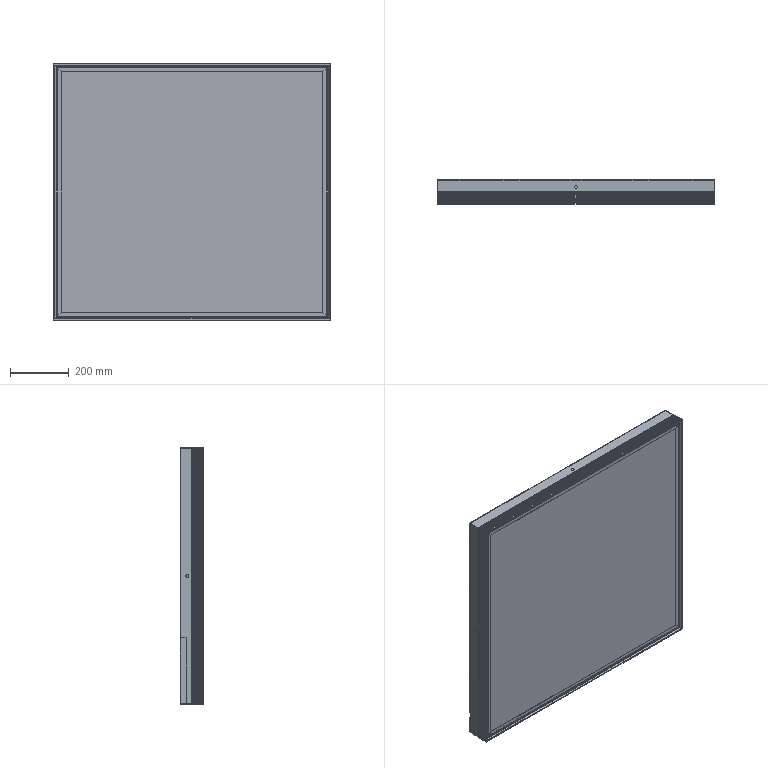Part | 41 solids | 2756 faces | box 940 x 80 x 870 mm | volume 96306060 mm3 | plane 1766 | cylinder 890 | spline 100 | commonest cylinder face diameters 7 x330 0.4 x156 11 x118 2.4 x104 4.2 x80 2 x38